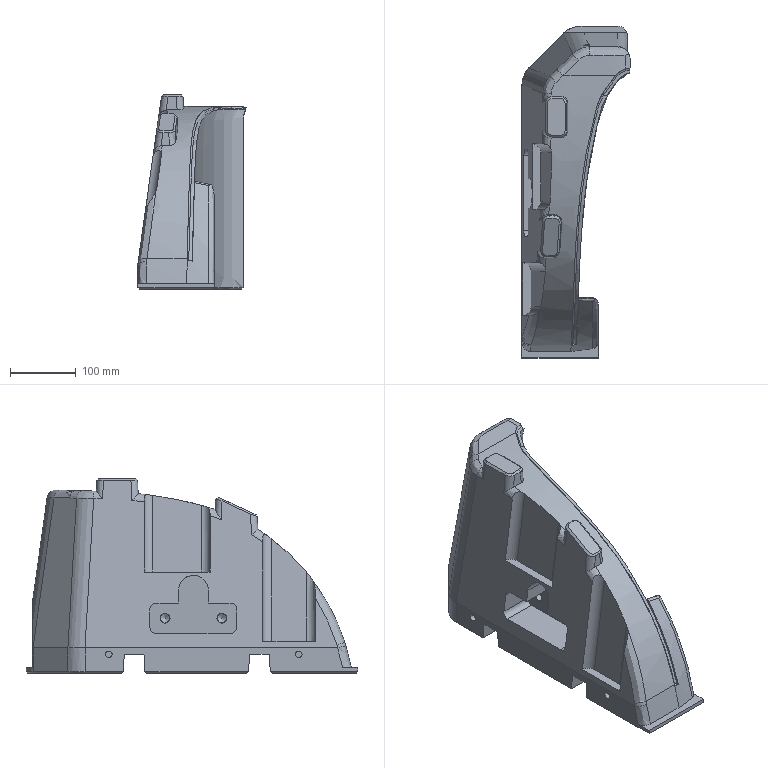Part | STEP file | solid 41 | 1 solid | 166 faces | box 164.037 x 503.365 x 295.607 mm | volume 9582610 mm3 | spline 81 | plane 39 | cylinder 34 | other 8 | cone 4 | commonest cylinder face diameters 10 x11 20 x6 18 x4 26 x4 74 x4 14 x2